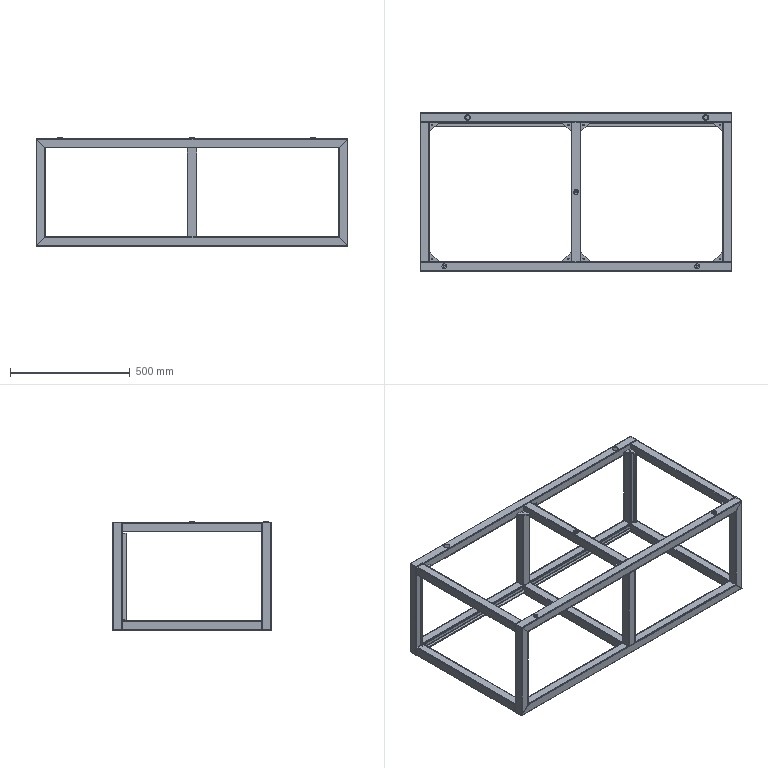Part | SolidWorks | 31 solids | 455 faces | box 1300 x 660 x 453 mm | volume 3352763 mm3 | plane 257 | cylinder 198 | commonest cylinder face diameters 2 x64 6 x64 16 x22 5 x16 6.5 x8 8.5 x6